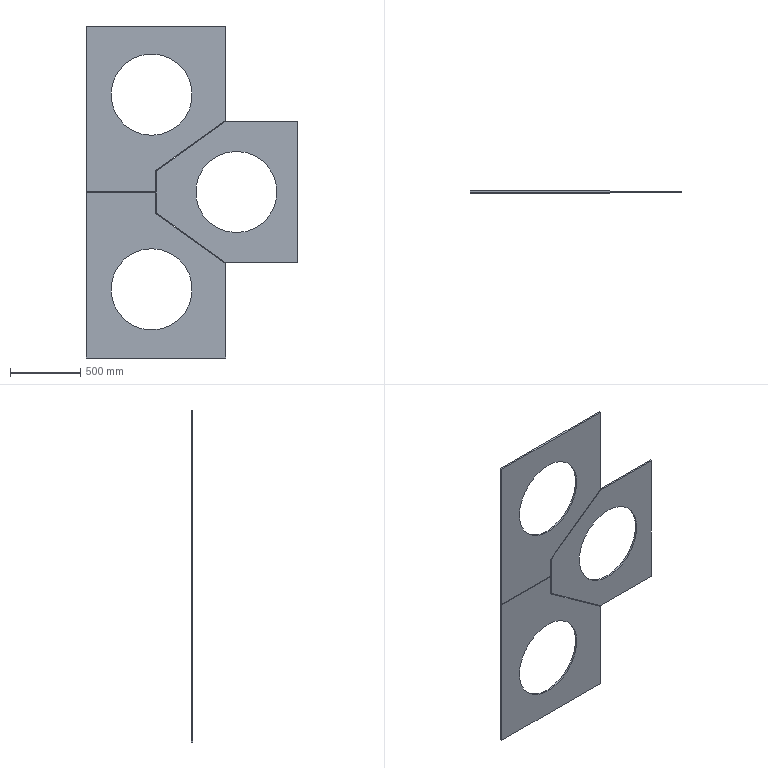Part | STEP file | Metering pad plate 2 | 3 solids | 30 faces | box 1510 x 12 x 2370 mm | volume 24906794 mm3 | plane 24 | cylinder 6 | commonest cylinder face diameters 580 x6